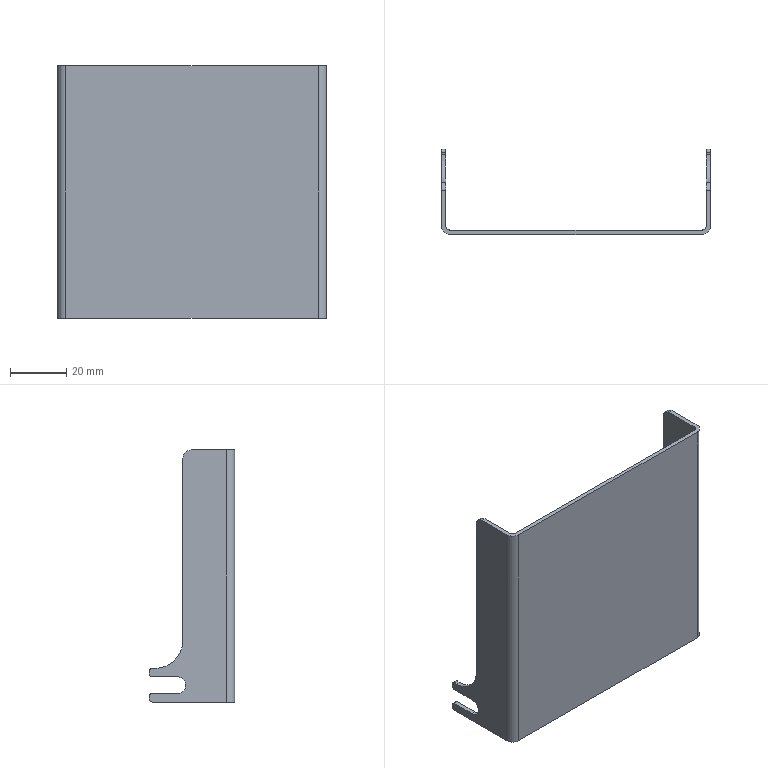Part | NX | features BREP 1 | 1 solid | 38 faces | box 96 x 30.5 x 90 mm | volume 17555 mm3 | plane 20 | cylinder 18 | commonest cylinder face diameters 2 x8 6 x6 3 x2 20 x2
STEP:
#1=CARTESIAN_POINT('',(-45.,0.,90.));
#2=VERTEX_POINT('',#1);
#3=CARTESIAN_POINT('',(45.,0.,90.));
#4=VERTEX_POINT('',#3);
#5=CARTESIAN_POINT('',(-46.5,0.,90.));
#6=DIRECTION('',(1.,0.,0.));
#7=VECTOR('',#6,1000.);
#8=LINE('',#5,#7);
#9=EDGE_CURVE('',#2,#4,#8,.T.);
#10=ORIENTED_EDGE('',*,*,#9,.T.);
#11=CARTESIAN_POINT('',(45.,0.,0.));
#12=VERTEX_POINT('',#11);
#13=CARTESIAN_POINT('',(45.,0.,90.));
#14=DIRECTION('',(0.,0.,-1.));
#15=VECTOR('',#14,1000.);
#16=LINE('',#13,#15);
#17=EDGE_CURVE('',#4,#12,#16,.T.);
#18=ORIENTED_EDGE('',*,*,#17,.T.);
#19=CARTESIAN_POINT('',(-45.,0.,0.));
#20=VERTEX_POINT('',#19);
#21=CARTESIAN_POINT('',(-46.5,0.,0.));
#22=DIRECTION('',(-1.,0.,0.));
#23=VECTOR('',#22,1000.);
#24=LINE('',#21,#23);
#25=EDGE_CURVE('',#12,#20,#24,.T.);
#26=ORIENTED_EDGE('',*,*,#25,.T.);
#27=CARTESIAN_POINT('',(-45.,0.,90.));
#28=DIRECTION('',(0.,0.,1.));
#29=VECTOR('',#28,1000.);
#30=LINE('',#27,#29);
#31=EDGE_CURVE('',#20,#2,#30,.T.);
#32=ORIENTED_EDGE('',*,*,#31,.T.);
#33=EDGE_LOOP('',(#10,#18,#26,#32));
#34=FACE_BOUND('',#33,.T.);
#35=CARTESIAN_POINT('',(-46.5,0.,90.));
#36=DIRECTION('',(0.,1.,0.));
#37=DIRECTION('',(1.,0.,0.));
#38=AXIS2_PLACEMENT_3D('',#35,#36,#37);
#39=PLANE('',#38);
#40=ADVANCED_FACE('',(#34),#39,.T.);
#41=ORIENTED_EDGE('',*,*,#17,.F.);
#42=CARTESIAN_POINT('',(46.5,1.5,90.));
#43=VERTEX_POINT('',#42);
#44=CARTESIAN_POINT('',(45.,1.5,90.));
#45=DIRECTION('',(0.,0.,-1.));
#46=DIRECTION('',(-1.,0.,0.));
#47=AXIS2_PLACEMENT_3D('',#44,#45,#46);
#48=CIRCLE('',#47,1.5);
#49=EDGE_CURVE('',#43,#4,#48,.T.);
#50=ORIENTED_EDGE('',*,*,#49,.F.);
#51=CARTESIAN_POINT('',(46.5,1.5,0.));
#52=VERTEX_POINT('',#51);
#53=CARTESIAN_POINT('',(46.5,1.5,90.));
#54=DIRECTION('',(0.,0.,1.));
#55=VECTOR('',#54,1000.);
#56=LINE('',#53,#55);
#57=EDGE_CURVE('',#52,#43,#56,.T.);
#58=ORIENTED_EDGE('',*,*,#57,.F.);
#59=CARTESIAN_POINT('',(45.,1.5,0.));
#60=DIRECTION('',(0.,0.,1.));
#61=DIRECTION('',(-1.,0.,0.));
#62=AXIS2_PLACEMENT_3D('',#59,#60,#61);
#63=CIRCLE('',#62,1.5);
#64=EDGE_CURVE('',#12,#52,#63,.T.);
#65=ORIENTED_EDGE('',*,*,#64,.F.);
#66=EDGE_LOOP('',(#41,#50,#58,#65));
#67=FACE_BOUND('',#66,.T.);
#68=CARTESIAN_POINT('',(45.,1.5,90.));
#69=DIRECTION('',(0.,0.,-1.));
#70=DIRECTION('',(1.,0.,0.));
#71=AXIS2_PLACEMENT_3D('',#68,#69,#70);
#72=CYLINDRICAL_SURFACE('',#71,1.5);
#73=ADVANCED_FACE('',(#67),#72,.F.);
#74=CARTESIAN_POINT('',(-45.,-1.5,90.));
#75=VERTEX_POINT('',#74);
#76=CARTESIAN_POINT('',(45.,-1.5,90.));
#77=VERTEX_POINT('',#76);
#78=CARTESIAN_POINT('',(-48.,-1.5,90.));
#79=DIRECTION('',(1.,0.,0.));
#80=VECTOR('',#79,1000.);
#81=LINE('',#78,#80);
#82=EDGE_CURVE('',#75,#77,#81,.T.);
#83=ORIENTED_EDGE('',*,*,#82,.T.);
#84=CARTESIAN_POINT('',(48.,1.5,90.));
#85=VERTEX_POINT('',#84);
#86=CARTESIAN_POINT('',(45.,1.5,90.));
#87=DIRECTION('',(0.,0.,1.));
#88=DIRECTION('',(-1.,0.,0.));
#89=AXIS2_PLACEMENT_3D('',#86,#87,#88);
#90=CIRCLE('',#89,3.);
#91=EDGE_CURVE('',#77,#85,#90,.T.);
#92=ORIENTED_EDGE('',*,*,#91,.T.);
#93=CARTESIAN_POINT('',(48.,14.,90.));
#94=VERTEX_POINT('',#93);
#95=CARTESIAN_POINT('',(48.,-1.5,90.));
#96=DIRECTION('',(0.,1.,0.));
#97=VECTOR('',#96,1000.);
#98=LINE('',#95,#97);
#99=EDGE_CURVE('',#85,#94,#98,.T.);
#100=ORIENTED_EDGE('',*,*,#99,.T.);
#101=CARTESIAN_POINT('',(46.5,14.,90.));
#102=VERTEX_POINT('',#101);
#103=CARTESIAN_POINT('',(46.5,14.,90.));
#104=DIRECTION('',(1.,0.,0.));
#105=VECTOR('',#104,1000.);
#106=LINE('',#103,#105);
#107=EDGE_CURVE('',#102,#94,#106,.T.);
#108=ORIENTED_EDGE('',*,*,#107,.F.);
#109=CARTESIAN_POINT('',(46.5,0.,90.));
#110=DIRECTION('',(0.,1.,0.));
#111=VECTOR('',#110,1000.);
#112=LINE('',#109,#111);
#113=EDGE_CURVE('',#43,#102,#112,.T.);
#114=ORIENTED_EDGE('',*,*,#113,.F.);
#115=ORIENTED_EDGE('',*,*,#49,.T.);
#116=ORIENTED_EDGE('',*,*,#9,.F.);
#117=CARTESIAN_POINT('',(-46.5,1.5,90.));
#118=VERTEX_POINT('',#117);
#119=CARTESIAN_POINT('',(-45.,1.5,90.));
#120=DIRECTION('',(0.,0.,-1.));
#121=DIRECTION('',(-1.,0.,0.));
#122=AXIS2_PLACEMENT_3D('',#119,#120,#121);
#123=CIRCLE('',#122,1.5);
#124=EDGE_CURVE('',#2,#118,#123,.T.);
#125=ORIENTED_EDGE('',*,*,#124,.T.);
#126=CARTESIAN_POINT('',(-46.5,14.,90.));
#127=VERTEX_POINT('',#126);
#128=CARTESIAN_POINT('',(-46.5,17.,90.));
#129=DIRECTION('',(0.,-1.,0.));
#130=VECTOR('',#129,1000.);
#131=LINE('',#128,#130);
#132=EDGE_CURVE('',#127,#118,#131,.T.);
#133=ORIENTED_EDGE('',*,*,#132,.F.);
#134=CARTESIAN_POINT('',(-48.,14.,90.));
#135=VERTEX_POINT('',#134);
#136=CARTESIAN_POINT('',(45.,14.,90.));
#137=DIRECTION('',(1.,0.,0.));
#138=VECTOR('',#137,1000.);
#139=LINE('',#136,#138);
#140=EDGE_CURVE('',#135,#127,#139,.T.);
#141=ORIENTED_EDGE('',*,*,#140,.F.);
#142=CARTESIAN_POINT('',(-48.,1.5,90.));
#143=VERTEX_POINT('',#142);
#144=CARTESIAN_POINT('',(-48.,1.5,90.));
#145=DIRECTION('',(0.,1.,0.));
#146=VECTOR('',#145,1000.);
#147=LINE('',#144,#146);
#148=EDGE_CURVE('',#143,#135,#147,.T.);
#149=ORIENTED_EDGE('',*,*,#148,.F.);
#150=CARTESIAN_POINT('',(-45.,1.5,90.));
#151=DIRECTION('',(0.,0.,1.));
#152=DIRECTION('',(-1.,0.,0.));
#153=AXIS2_PLACEMENT_3D('',#150,#151,#152);
#154=CIRCLE('',#153,3.);
#155=EDGE_CURVE('',#143,#75,#154,.T.);
#156=ORIENTED_EDGE('',*,*,#155,.T.);
#157=EDGE_LOOP('',(#83,#92,#100,#108,#114,#115,#116,#125,#133,#141,#149,#156));
#158=FACE_BOUND('',#157,.T.);
#159=CARTESIAN_POINT('',(-48.,1.5,90.));
#160=DIRECTION('',(0.,0.,1.));
#161=DIRECTION('',(-1.,0.,0.));
#162=AXIS2_PLACEMENT_3D('',#159,#160,#161);
#163=PLANE('',#162);
#164=ADVANCED_FACE('',(#158),#163,.T.);
#165=CARTESIAN_POINT('',(-46.5,1.5,0.));
#166=VERTEX_POINT('',#165);
#167=CARTESIAN_POINT('',(-46.5,1.5,90.));
#168=DIRECTION('',(0.,0.,-1.));
#169=VECTOR('',#168,1000.);
#170=LINE('',#167,#169);
#171=EDGE_CURVE('',#118,#166,#170,.T.);
#172=ORIENTED_EDGE('',*,*,#171,.F.);
#173=ORIENTED_EDGE('',*,*,#124,.F.);
#174=ORIENTED_EDGE('',*,*,#31,.F.);
#175=CARTESIAN_POINT('',(-45.,1.5,0.));
#176=DIRECTION('',(0.,0.,1.));
#177=DIRECTION('',(-1.,0.,0.));
#178=AXIS2_PLACEMENT_3D('',#175,#176,#177);
#179=CIRCLE('',#178,1.5);
#180=EDGE_CURVE('',#166,#20,#179,.T.);
#181=ORIENTED_EDGE('',*,*,#180,.F.);
#182=EDGE_LOOP('',(#172,#173,#174,#181));
#183=FACE_BOUND('',#182,.T.);
#184=CARTESIAN_POINT('',(-45.,1.5,90.));
#185=DIRECTION('',(0.,0.,-1.));
#186=DIRECTION('',(1.,0.,0.));
#187=AXIS2_PLACEMENT_3D('',#184,#185,#186);
#188=CYLINDRICAL_SURFACE('',#187,1.5);
#189=ADVANCED_FACE('',(#183),#188,.F.);
#190=CARTESIAN_POINT('',(45.,-1.5,0.));
#191=VERTEX_POINT('',#190);
#192=CARTESIAN_POINT('',(-45.,-1.5,0.));
#193=VERTEX_POINT('',#192);
#194=CARTESIAN_POINT('',(48.,-1.5,0.));
#195=DIRECTION('',(-1.,0.,0.));
#196=VECTOR('',#195,1000.);
#197=LINE('',#194,#196);
#198=EDGE_CURVE('',#191,#193,#197,.T.);
#199=ORIENTED_EDGE('',*,*,#198,.T.);
#200=CARTESIAN_POINT('',(-48.,1.5,0.));
#201=VERTEX_POINT('',#200);
#202=CARTESIAN_POINT('',(-45.,1.5,0.));
#203=DIRECTION('',(0.,0.,-1.));
#204=DIRECTION('',(-1.,0.,0.));
#205=AXIS2_PLACEMENT_3D('',#202,#203,#204);
#206=CIRCLE('',#205,3.);
#207=EDGE_CURVE('',#193,#201,#206,.T.);
#208=ORIENTED_EDGE('',*,*,#207,.T.);
#209=CARTESIAN_POINT('',(-48.,28.,0.));
#210=VERTEX_POINT('',#209);
#211=CARTESIAN_POINT('',(-48.,-1.5,0.));
#212=DIRECTION('',(0.,1.,0.));
#213=VECTOR('',#212,1000.);
#214=LINE('',#211,#213);
#215=EDGE_CURVE('',#201,#210,#214,.T.);
#216=ORIENTED_EDGE('',*,*,#215,.T.);
#217=CARTESIAN_POINT('',(-46.5,28.,0.));
#218=VERTEX_POINT('',#217);
#219=CARTESIAN_POINT('',(-29.529,28.,0.));
#220=DIRECTION('',(-1.,0.,0.));
#221=VECTOR('',#220,1000.);
#222=LINE('',#219,#221);
#223=EDGE_CURVE('',#218,#210,#222,.T.);
#224=ORIENTED_EDGE('',*,*,#223,.F.);
#225=CARTESIAN_POINT('',(-46.5,17.,0.));
#226=DIRECTION('',(0.,1.,0.));
#227=VECTOR('',#226,1000.);
#228=LINE('',#225,#227);
#229=EDGE_CURVE('',#166,#218,#228,.T.);
#230=ORIENTED_EDGE('',*,*,#229,.F.);
#231=ORIENTED_EDGE('',*,*,#180,.T.);
#232=ORIENTED_EDGE('',*,*,#25,.F.);
#233=ORIENTED_EDGE('',*,*,#64,.T.);
#234=CARTESIAN_POINT('',(46.5,28.,0.));
#235=VERTEX_POINT('',#234);
#236=CARTESIAN_POINT('',(46.5,0.,0.));
#237=DIRECTION('',(0.,-1.,0.));
#238=VECTOR('',#237,1000.);
#239=LINE('',#236,#238);
#240=EDGE_CURVE('',#235,#52,#239,.T.);
#241=ORIENTED_EDGE('',*,*,#240,.F.);
#242=CARTESIAN_POINT('',(48.,28.,0.));
#243=VERTEX_POINT('',#242);
#244=CARTESIAN_POINT('',(45.,28.,0.));
#245=DIRECTION('',(1.,0.,0.));
#246=VECTOR('',#245,1000.);
#247=LINE('',#244,#246);
#248=EDGE_CURVE('',#235,#243,#247,.T.);
#249=ORIENTED_EDGE('',*,*,#248,.T.);
#250=CARTESIAN_POINT('',(48.,1.5,0.));
#251=VERTEX_POINT('',#250);
#252=CARTESIAN_POINT('',(48.,1.5,0.));
#253=DIRECTION('',(0.,-1.,0.));
#254=VECTOR('',#253,1000.);
#255=LINE('',#252,#254);
#256=EDGE_CURVE('',#243,#251,#255,.T.);
#257=ORIENTED_EDGE('',*,*,#256,.T.);
#258=CARTESIAN_POINT('',(45.,1.5,0.));
#259=DIRECTION('',(0.,0.,-1.));
#260=DIRECTION('',(-1.,0.,0.));
#261=AXIS2_PLACEMENT_3D('',#258,#259,#260);
#262=CIRCLE('',#261,3.);
#263=EDGE_CURVE('',#251,#191,#262,.T.);
#264=ORIENTED_EDGE('',*,*,#263,.T.);
#265=EDGE_LOOP('',(#199,#208,#216,#224,#230,#231,#232,#233,#241,#249,#257,#264));
#266=FACE_BOUND('',#265,.T.);
#267=CARTESIAN_POINT('',(48.,1.5,0.));
#268=DIRECTION('',(0.,0.,-1.));
#269=DIRECTION('',(1.,0.,0.));
#270=AXIS2_PLACEMENT_3D('',#267,#268,#269);
#271=PLANE('',#270);
#272=ADVANCED_FACE('',(#266),#271,.T.);
#273=CARTESIAN_POINT('',(46.5,27.,12.));
#274=VERTEX_POINT('',#273);
#275=CARTESIAN_POINT('',(46.5,28.,12.));
#276=VERTEX_POINT('',#275);
#277=CARTESIAN_POINT('',(46.5,0.,12.));
#278=DIRECTION('',(0.,1.,0.));
#279=VECTOR('',#278,1000.);
#280=LINE('',#277,#279);
#281=EDGE_CURVE('',#274,#276,#280,.T.);
#282=ORIENTED_EDGE('',*,*,#281,.T.);
#283=CARTESIAN_POINT('',(46.5,29.,11.));
#284=VERTEX_POINT('',#283);
#285=CARTESIAN_POINT('',(46.5,28.,11.));
#286=DIRECTION('',(-1.,0.,0.));
#287=DIRECTION('',(0.,0.,-1.));
#288=AXIS2_PLACEMENT_3D('',#285,#286,#287);
#289=CIRCLE('',#288,1.);
#290=EDGE_CURVE('',#276,#284,#289,.T.);
#291=ORIENTED_EDGE('',*,*,#290,.T.);
#292=CARTESIAN_POINT('',(46.5,29.,10.));
#293=VERTEX_POINT('',#292);
#294=CARTESIAN_POINT('',(46.5,29.,90.));
#295=DIRECTION('',(0.,0.,-1.));
#296=VECTOR('',#295,1000.);
#297=LINE('',#294,#296);
#298=EDGE_CURVE('',#284,#293,#297,.T.);
#299=ORIENTED_EDGE('',*,*,#298,.T.);
#300=CARTESIAN_POINT('',(46.5,28.,9.));
#301=VERTEX_POINT('',#300);
#302=CARTESIAN_POINT('',(46.5,28.,10.));
#303=DIRECTION('',(-1.,0.,0.));
#304=DIRECTION('',(0.,0.,1.));
#305=AXIS2_PLACEMENT_3D('',#302,#303,#304);
#306=CIRCLE('',#305,1.);
#307=EDGE_CURVE('',#293,#301,#306,.T.);
#308=ORIENTED_EDGE('',*,*,#307,.T.);
#309=CARTESIAN_POINT('',(46.5,19.,9.));
#310=VERTEX_POINT('',#309);
#311=CARTESIAN_POINT('',(46.5,0.,9.));
#312=DIRECTION('',(0.,-1.,0.));
#313=VECTOR('',#312,1000.);
#314=LINE('',#311,#313);
#315=EDGE_CURVE('',#301,#310,#314,.T.);
#316=ORIENTED_EDGE('',*,*,#315,.T.);
#317=CARTESIAN_POINT('',(46.5,19.,3.));
#318=VERTEX_POINT('',#317);
#319=CARTESIAN_POINT('',(46.5,19.,6.));
#320=DIRECTION('',(1.,0.,0.));
#321=DIRECTION('',(0.,0.,-1.));
#322=AXIS2_PLACEMENT_3D('',#319,#320,#321);
#323=CIRCLE('',#322,3.);
#324=EDGE_CURVE('',#310,#318,#323,.T.);
#325=ORIENTED_EDGE('',*,*,#324,.T.);
#326=CARTESIAN_POINT('',(46.5,28.,3.));
#327=VERTEX_POINT('',#326);
#328=CARTESIAN_POINT('',(46.5,0.,3.));
#329=DIRECTION('',(0.,1.,0.));
#330=VECTOR('',#329,1000.);
#331=LINE('',#328,#330);
#332=EDGE_CURVE('',#318,#327,#331,.T.);
#333=ORIENTED_EDGE('',*,*,#332,.T.);
#334=CARTESIAN_POINT('',(46.5,29.,2.));
#335=VERTEX_POINT('',#334);
#336=CARTESIAN_POINT('',(46.5,28.,2.));
#337=DIRECTION('',(-1.,0.,0.));
#338=DIRECTION('',(0.,0.,-1.));
#339=AXIS2_PLACEMENT_3D('',#336,#337,#338);
#340=CIRCLE('',#339,1.);
#341=EDGE_CURVE('',#327,#335,#340,.T.);
#342=ORIENTED_EDGE('',*,*,#341,.T.);
#343=CARTESIAN_POINT('',(46.5,29.,1.));
#344=VERTEX_POINT('',#343);
#345=CARTESIAN_POINT('',(46.5,29.,90.));
#346=DIRECTION('',(0.,0.,-1.));
#347=VECTOR('',#346,1000.);
#348=LINE('',#345,#347);
#349=EDGE_CURVE('',#335,#344,#348,.T.);
#350=ORIENTED_EDGE('',*,*,#349,.T.);
#351=CARTESIAN_POINT('',(46.5,28.,1.));
#352=DIRECTION('',(-1.,0.,0.));
#353=DIRECTION('',(0.,0.,-1.));
#354=AXIS2_PLACEMENT_3D('',#351,#352,#353);
#355=CIRCLE('',#354,1.);
#356=EDGE_CURVE('',#344,#235,#355,.T.);
#357=ORIENTED_EDGE('',*,*,#356,.T.);
#358=ORIENTED_EDGE('',*,*,#240,.T.);
#359=ORIENTED_EDGE('',*,*,#57,.T.);
#360=ORIENTED_EDGE('',*,*,#113,.T.);
#361=CARTESIAN_POINT('',(46.5,17.,87.));
#362=VERTEX_POINT('',#361);
#363=CARTESIAN_POINT('',(46.5,14.,87.));
#364=DIRECTION('',(-1.,0.,0.));
#365=DIRECTION('',(0.,0.,-1.));
#366=AXIS2_PLACEMENT_3D('',#363,#364,#365);
#367=CIRCLE('',#366,3.);
#368=EDGE_CURVE('',#102,#362,#367,.T.);
#369=ORIENTED_EDGE('',*,*,#368,.T.);
#370=CARTESIAN_POINT('',(46.5,17.,22.));
#371=VERTEX_POINT('',#370);
#372=CARTESIAN_POINT('',(46.5,17.,90.));
#373=DIRECTION('',(0.,0.,-1.));
#374=VECTOR('',#373,1000.);
#375=LINE('',#372,#374);
#376=EDGE_CURVE('',#362,#371,#375,.T.);
#377=ORIENTED_EDGE('',*,*,#376,.T.);
#378=CARTESIAN_POINT('',(46.5,27.,22.));
#379=DIRECTION('',(1.,0.,0.));
#380=DIRECTION('',(0.,0.,1.));
#381=AXIS2_PLACEMENT_3D('',#378,#379,#380);
#382=CIRCLE('',#381,10.);
#383=EDGE_CURVE('',#371,#274,#382,.T.);
#384=ORIENTED_EDGE('',*,*,#383,.T.);
#385=EDGE_LOOP('',(#282,#291,#299,#308,#316,#325,#333,#342,#350,#357,#358,#359,#360,#369,#377,#384));
#386=FACE_BOUND('',#385,.T.);
#387=CARTESIAN_POINT('',(46.5,0.,90.));
#388=DIRECTION('',(-1.,0.,0.));
#389=DIRECTION('',(0.,0.,-1.));
#390=AXIS2_PLACEMENT_3D('',#387,#388,#389);
#391=PLANE('',#390);
#392=ADVANCED_FACE('',(#386),#391,.T.);
#393=CARTESIAN_POINT('',(45.,-1.5,90.));
#394=DIRECTION('',(0.,0.,-1.));
#395=VECTOR('',#394,1000.);
#396=LINE('',#393,#395);
#397=EDGE_CURVE('',#77,#191,#396,.T.);
#398=ORIENTED_EDGE('',*,*,#397,.F.);
#399=ORIENTED_EDGE('',*,*,#82,.F.);
#400=CARTESIAN_POINT('',(-45.,-1.5,90.));
#401=DIRECTION('',(0.,0.,1.));
#402=VECTOR('',#401,1000.);
#403=LINE('',#400,#402);
#404=EDGE_CURVE('',#193,#75,#403,.T.);
#405=ORIENTED_EDGE('',*,*,#404,.F.);
#406=ORIENTED_EDGE('',*,*,#198,.F.);
#407=EDGE_LOOP('',(#398,#399,#405,#406));
#408=FACE_BOUND('',#407,.T.);
#409=CARTESIAN_POINT('',(-46.5,-1.5,90.));
#410=DIRECTION('',(0.,1.,0.));
#411=DIRECTION('',(1.,0.,0.));
#412=AXIS2_PLACEMENT_3D('',#409,#410,#411);
#413=PLANE('',#412);
#414=ADVANCED_FACE('',(#408),#413,.F.);
#415=ORIENTED_EDGE('',*,*,#229,.T.);
#416=CARTESIAN_POINT('',(-46.5,29.,1.));
#417=VERTEX_POINT('',#416);
#418=CARTESIAN_POINT('',(-46.5,28.,1.));
#419=DIRECTION('',(1.,0.,0.));
#420=DIRECTION('',(0.,0.,1.));
#421=AXIS2_PLACEMENT_3D('',#418,#419,#420);
#422=CIRCLE('',#421,1.);
#423=EDGE_CURVE('',#218,#417,#422,.T.);
#424=ORIENTED_EDGE('',*,*,#423,.T.);
#425=CARTESIAN_POINT('',(-46.5,29.,2.));
#426=VERTEX_POINT('',#425);
#427=CARTESIAN_POINT('',(-46.5,29.,90.));
#428=DIRECTION('',(0.,0.,1.));
#429=VECTOR('',#428,1000.);
#430=LINE('',#427,#429);
#431=EDGE_CURVE('',#417,#426,#430,.T.);
#432=ORIENTED_EDGE('',*,*,#431,.T.);
#433=CARTESIAN_POINT('',(-46.5,28.,3.));
#434=VERTEX_POINT('',#433);
#435=CARTESIAN_POINT('',(-46.5,28.,2.));
#436=DIRECTION('',(1.,0.,0.));
#437=DIRECTION('',(0.,0.,1.));
#438=AXIS2_PLACEMENT_3D('',#435,#436,#437);
#439=CIRCLE('',#438,1.);
#440=EDGE_CURVE('',#426,#434,#439,.T.);
#441=ORIENTED_EDGE('',*,*,#440,.T.);
#442=CARTESIAN_POINT('',(-46.5,19.,3.));
#443=VERTEX_POINT('',#442);
#444=CARTESIAN_POINT('',(-46.5,17.,3.));
#445=DIRECTION('',(0.,-1.,0.));
#446=VECTOR('',#445,1000.);
#447=LINE('',#444,#446);
#448=EDGE_CURVE('',#434,#443,#447,.T.);
#449=ORIENTED_EDGE('',*,*,#448,.T.);
#450=CARTESIAN_POINT('',(-46.5,19.,9.));
#451=VERTEX_POINT('',#450);
#452=CARTESIAN_POINT('',(-46.5,19.,6.));
#453=DIRECTION('',(-1.,0.,0.));
#454=DIRECTION('',(0.,0.,-1.));
#455=AXIS2_PLACEMENT_3D('',#452,#453,#454);
#456=CIRCLE('',#455,3.);
#457=EDGE_CURVE('',#443,#451,#456,.T.);
#458=ORIENTED_EDGE('',*,*,#457,.T.);
#459=CARTESIAN_POINT('',(-46.5,28.,9.));
#460=VERTEX_POINT('',#459);
#461=CARTESIAN_POINT('',(-46.5,17.,9.));
#462=DIRECTION('',(0.,1.,0.));
#463=VECTOR('',#462,1000.);
#464=LINE('',#461,#463);
#465=EDGE_CURVE('',#451,#460,#464,.T.);
#466=ORIENTED_EDGE('',*,*,#465,.T.);
#467=CARTESIAN_POINT('',(-46.5,29.,10.));
#468=VERTEX_POINT('',#467);
#469=CARTESIAN_POINT('',(-46.5,28.,10.));
#470=DIRECTION('',(1.,0.,0.));
#471=DIRECTION('',(0.,0.,1.));
#472=AXIS2_PLACEMENT_3D('',#469,#470,#471);
#473=CIRCLE('',#472,1.);
#474=EDGE_CURVE('',#460,#468,#473,.T.);
#475=ORIENTED_EDGE('',*,*,#474,.T.);
#476=CARTESIAN_POINT('',(-46.5,29.,11.));
#477=VERTEX_POINT('',#476);
#478=CARTESIAN_POINT('',(-46.5,29.,90.));
#479=DIRECTION('',(0.,0.,1.));
#480=VECTOR('',#479,1000.);
#481=LINE('',#478,#480);
#482=EDGE_CURVE('',#468,#477,#481,.T.);
#483=ORIENTED_EDGE('',*,*,#482,.T.);
#484=CARTESIAN_POINT('',(-46.5,28.,12.));
#485=VERTEX_POINT('',#484);
#486=CARTESIAN_POINT('',(-46.5,28.,11.));
#487=DIRECTION('',(1.,0.,0.));
#488=DIRECTION('',(0.,0.,1.));
#489=AXIS2_PLACEMENT_3D('',#486,#487,#488);
#490=CIRCLE('',#489,1.);
#491=EDGE_CURVE('',#477,#485,#490,.T.);
#492=ORIENTED_EDGE('',*,*,#491,.T.);
#493=CARTESIAN_POINT('',(-46.5,27.,12.));
#494=VERTEX_POINT('',#493);
#495=CARTESIAN_POINT('',(-46.5,17.,12.));
#496=DIRECTION('',(0.,-1.,0.));
#497=VECTOR('',#496,1000.);
#498=LINE('',#495,#497);
#499=EDGE_CURVE('',#485,#494,#498,.T.);
#500=ORIENTED_EDGE('',*,*,#499,.T.);
#501=CARTESIAN_POINT('',(-46.5,17.,22.));
#502=VERTEX_POINT('',#501);
#503=CARTESIAN_POINT('',(-46.5,27.,22.));
#504=DIRECTION('',(-1.,0.,0.));
#505=DIRECTION('',(0.,0.,-1.));
#506=AXIS2_PLACEMENT_3D('',#503,#504,#505);
#507=CIRCLE('',#506,10.);
#508=EDGE_CURVE('',#494,#502,#507,.T.);
#509=ORIENTED_EDGE('',*,*,#508,.T.);
#510=CARTESIAN_POINT('',(-46.5,17.,87.));
#511=VERTEX_POINT('',#510);
#512=CARTESIAN_POINT('',(-46.5,17.,90.));
#513=DIRECTION('',(0.,0.,1.));
#514=VECTOR('',#513,1000.);
#515=LINE('',#512,#514);
#516=EDGE_CURVE('',#502,#511,#515,.T.);
#517=ORIENTED_EDGE('',*,*,#516,.T.);
#518=CARTESIAN_POINT('',(-46.5,14.,87.));
#519=DIRECTION('',(1.,0.,0.));
#520=DIRECTION('',(0.,0.,1.));
#521=AXIS2_PLACEMENT_3D('',#518,#519,#520);
#522=CIRCLE('',#521,3.);
#523=EDGE_CURVE('',#511,#127,#522,.T.);
#524=ORIENTED_EDGE('',*,*,#523,.T.);
#525=ORIENTED_EDGE('',*,*,#132,.T.);
#526=ORIENTED_EDGE('',*,*,#171,.T.);
#527=EDGE_LOOP('',(#415,#424,#432,#441,#449,#458,#466,#475,#483,#492,#500,#509,#517,#524,#525,#526));
#528=FACE_BOUND('',#527,.T.);
#529=CARTESIAN_POINT('',(-46.5,17.,90.));
#530=DIRECTION('',(1.,0.,0.));
#531=DIRECTION('',(0.,0.,1.));
#532=AXIS2_PLACEMENT_3D('',#529,#530,#531);
#533=PLANE('',#532);
#534=ADVANCED_FACE('',(#528),#533,.T.);
#535=ORIENTED_EDGE('',*,*,#91,.F.);
#536=ORIENTED_EDGE('',*,*,#397,.T.);
#537=ORIENTED_EDGE('',*,*,#263,.F.);
#538=CARTESIAN_POINT('',(48.,1.5,90.));
#539=DIRECTION('',(0.,0.,1.));
#540=VECTOR('',#539,1000.);
#541=LINE('',#538,#540);
#542=EDGE_CURVE('',#251,#85,#541,.T.);
#543=ORIENTED_EDGE('',*,*,#542,.T.);
#544=EDGE_LOOP('',(#535,#536,#537,#543));
#545=FACE_BOUND('',#544,.T.);
#546=CARTESIAN_POINT('',(45.,1.5,90.));
#547=DIRECTION('',(0.,0.,-1.));
#548=DIRECTION('',(1.,0.,0.));
#549=AXIS2_PLACEMENT_3D('',#546,#547,#548);
#550=CYLINDRICAL_SURFACE('',#549,3.);
#551=ADVANCED_FACE('',(#545),#550,.T.);
#552=CARTESIAN_POINT('',(48.,28.,12.));
#553=VERTEX_POINT('',#552);
#554=CARTESIAN_POINT('',(48.,29.,11.));
#555=VERTEX_POINT('',#554);
#556=CARTESIAN_POINT('',(48.,28.,11.));
#557=DIRECTION('',(-1.,0.,0.));
#558=DIRECTION('',(0.,0.,-1.));
#559=AXIS2_PLACEMENT_3D('',#556,#557,#558);
#560=CIRCLE('',#559,1.);
#561=EDGE_CURVE('',#553,#555,#560,.T.);
#562=ORIENTED_EDGE('',*,*,#561,.T.);
#563=CARTESIAN_POINT('',(46.5,29.,11.));
#564=DIRECTION('',(-1.,0.,0.));
#565=VECTOR('',#564,1000.);
#566=LINE('',#563,#565);
#567=EDGE_CURVE('',#555,#284,#566,.T.);
#568=ORIENTED_EDGE('',*,*,#567,.T.);
#569=ORIENTED_EDGE('',*,*,#290,.F.);
#570=CARTESIAN_POINT('',(46.5,28.,12.));
#571=DIRECTION('',(1.,0.,0.));
#572=VECTOR('',#571,1000.);
#573=LINE('',#570,#572);
#574=EDGE_CURVE('',#276,#553,#573,.T.);
#575=ORIENTED_EDGE('',*,*,#574,.T.);
#576=EDGE_LOOP('',(#562,#568,#569,#575));
#577=FACE_BOUND('',#576,.T.);
#578=CARTESIAN_POINT('',(46.5,28.,11.));
#579=DIRECTION('',(1.,0.,0.));
#580=DIRECTION('',(0.,0.,1.));
#581=AXIS2_PLACEMENT_3D('',#578,#579,#580);
#582=CYLINDRICAL_SURFACE('',#581,1.);
#583=ADVANCED_FACE('',(#577),#582,.T.);
#584=ORIENTED_EDGE('',*,*,#281,.F.);
#585=CARTESIAN_POINT('',(48.,27.,12.));
#586=VERTEX_POINT('',#585);
#587=CARTESIAN_POINT('',(46.5,27.,12.));
#588=DIRECTION('',(1.,0.,0.));
#589=VECTOR('',#588,1000.);
#590=LINE('',#587,#589);
#591=EDGE_CURVE('',#274,#586,#590,.T.);
#592=ORIENTED_EDGE('',*,*,#591,.T.);
#593=CARTESIAN_POINT('',(48.,29.,12.));
#594=DIRECTION('',(0.,1.,0.));
#595=VECTOR('',#594,1000.);
#596=LINE('',#593,#595);
#597=EDGE_CURVE('',#586,#553,#596,.T.);
#598=ORIENTED_EDGE('',*,*,#597,.T.);
#599=ORIENTED_EDGE('',*,*,#574,.F.);
#600=EDGE_LOOP('',(#584,#592,#598,#599));
#601=FACE_BOUND('',#600,.T.);
#602=CARTESIAN_POINT('',(46.5,29.,12.));
#603=DIRECTION('',(0.,0.,1.));
#604=DIRECTION('',(0.,1.,0.));
#605=AXIS2_PLACEMENT_3D('',#602,#603,#604);
#606=PLANE('',#605);
#607=ADVANCED_FACE('',(#601),#606,.T.);
#608=CARTESIAN_POINT('',(48.,17.,22.));
#609=VERTEX_POINT('',#608);
#610=CARTESIAN_POINT('',(46.5,17.,22.));
#611=DIRECTION('',(-1.,0.,0.));
#612=VECTOR('',#611,1000.);
#613=LINE('',#610,#612);
#614=EDGE_CURVE('',#609,#371,#613,.T.);
#615=ORIENTED_EDGE('',*,*,#614,.F.);
#616=CARTESIAN_POINT('',(48.,27.,22.));
#617=DIRECTION('',(-1.,0.,0.));
#618=DIRECTION('',(0.,0.,1.));
#619=AXIS2_PLACEMENT_3D('',#616,#617,#618);
#620=CIRCLE('',#619,10.);
#621=EDGE_CURVE('',#586,#609,#620,.T.);
#622=ORIENTED_EDGE('',*,*,#621,.F.);
#623=ORIENTED_EDGE('',*,*,#591,.F.);
#624=ORIENTED_EDGE('',*,*,#383,.F.);
#625=EDGE_LOOP('',(#615,#622,#623,#624));
#626=FACE_BOUND('',#625,.T.);
#627=CARTESIAN_POINT('',(46.5,27.,22.));
#628=DIRECTION('',(-1.,0.,0.));
#629=DIRECTION('',(0.,0.,-1.));
#630=AXIS2_PLACEMENT_3D('',#627,#628,#629);
#631=CYLINDRICAL_SURFACE('',#630,10.);
#632=ADVANCED_FACE('',(#626),#631,.F.);
#633=CARTESIAN_POINT('',(48.,17.,87.));
#634=VERTEX_POINT('',#633);
#635=CARTESIAN_POINT('',(48.,17.,90.));
#636=DIRECTION('',(0.,0.,-1.));
#637=VECTOR('',#636,1000.);
#638=LINE('',#635,#637);
#639=EDGE_CURVE('',#634,#609,#638,.T.);
#640=ORIENTED_EDGE('',*,*,#639,.T.);
#641=ORIENTED_EDGE('',*,*,#614,.T.);
#642=ORIENTED_EDGE('',*,*,#376,.F.);
#643=CARTESIAN_POINT('',(46.5,17.,87.));
#644=DIRECTION('',(1.,0.,0.));
#645=VECTOR('',#644,1000.);
#646=LINE('',#643,#645);
#647=EDGE_CURVE('',#362,#634,#646,.T.);
#648=ORIENTED_EDGE('',*,*,#647,.T.);
#649=EDGE_LOOP('',(#640,#641,#642,#648));
#650=FACE_BOUND('',#649,.T.);
#651=CARTESIAN_POINT('',(46.5,17.,90.));
#652=DIRECTION('',(0.,1.,0.));
#653=DIRECTION('',(0.,0.,-1.));
#654=AXIS2_PLACEMENT_3D('',#651,#652,#653);
#655=PLANE('',#654);
#656=ADVANCED_FACE('',(#650),#655,.T.);
#657=CARTESIAN_POINT('',(48.,14.,87.));
#658=DIRECTION('',(-1.,0.,0.));
#659=DIRECTION('',(0.,0.,-1.));
#660=AXIS2_PLACEMENT_3D('',#657,#658,#659);
#661=CIRCLE('',#660,3.);
#662=EDGE_CURVE('',#94,#634,#661,.T.);
#663=ORIENTED_EDGE('',*,*,#662,.T.);
#664=ORIENTED_EDGE('',*,*,#647,.F.);
#665=ORIENTED_EDGE('',*,*,#368,.F.);
#666=ORIENTED_EDGE('',*,*,#107,.T.);
#667=EDGE_LOOP('',(#663,#664,#665,#666));
#668=FACE_BOUND('',#667,.T.);
#669=CARTESIAN_POINT('',(46.5,14.,87.));
#670=DIRECTION('',(1.,0.,0.));
#671=DIRECTION('',(0.,0.,1.));
#672=AXIS2_PLACEMENT_3D('',#669,#670,#671);
#673=CYLINDRICAL_SURFACE('',#672,3.);
#674=ADVANCED_FACE('',(#668),#673,.T.);
#675=CARTESIAN_POINT('',(48.,29.,1.));
#676=VERTEX_POINT('',#675);
#677=CARTESIAN_POINT('',(48.,28.,1.));
#678=DIRECTION('',(-1.,0.,0.));
#679=DIRECTION('',(0.,0.,-1.));
#680=AXIS2_PLACEMENT_3D('',#677,#678,#679);
#681=CIRCLE('',#680,1.);
#682=EDGE_CURVE('',#676,#243,#681,.T.);
#683=ORIENTED_EDGE('',*,*,#682,.T.);
#684=ORIENTED_EDGE('',*,*,#248,.F.);
#685=ORIENTED_EDGE('',*,*,#356,.F.);
#686=CARTESIAN_POINT('',(45.,29.,1.));
#687=DIRECTION('',(1.,0.,0.));
#688=VECTOR('',#687,1000.);
#689=LINE('',#686,#688);
#690=EDGE_CURVE('',#344,#676,#689,.T.);
#691=ORIENTED_EDGE('',*,*,#690,.T.);
#692=EDGE_LOOP('',(#683,#684,#685,#691));
#693=FACE_BOUND('',#692,.T.);
#694=CARTESIAN_POINT('',(45.,28.,1.));
#695=DIRECTION('',(1.,0.,0.));
#696=DIRECTION('',(0.,0.,1.));
#697=AXIS2_PLACEMENT_3D('',#694,#695,#696);
#698=CYLINDRICAL_SURFACE('',#697,1.);
#699=ADVANCED_FACE('',(#693),#698,.T.);
#700=CARTESIAN_POINT('',(48.,29.,2.));
#701=VERTEX_POINT('',#700);
#702=CARTESIAN_POINT('',(48.,29.,0.));
#703=DIRECTION('',(0.,0.,-1.));
#704=VECTOR('',#703,1000.);
#705=LINE('',#702,#704);
#706=EDGE_CURVE('',#701,#676,#705,.T.);
#707=ORIENTED_EDGE('',*,*,#706,.T.);
#708=ORIENTED_EDGE('',*,*,#690,.F.);
#709=ORIENTED_EDGE('',*,*,#349,.F.);
#710=CARTESIAN_POINT('',(46.5,29.,2.));
#711=DIRECTION('',(1.,0.,0.));
#712=VECTOR('',#711,1000.);
#713=LINE('',#710,#712);
#714=EDGE_CURVE('',#335,#701,#713,.T.);
#715=ORIENTED_EDGE('',*,*,#714,.T.);
#716=EDGE_LOOP('',(#707,#708,#709,#715));
#717=FACE_BOUND('',#716,.T.);
#718=CARTESIAN_POINT('',(46.5,29.,0.));
#719=DIRECTION('',(0.,1.,0.));
#720=DIRECTION('',(0.,0.,-1.));
#721=AXIS2_PLACEMENT_3D('',#718,#719,#720);
#722=PLANE('',#721);
#723=ADVANCED_FACE('',(#717),#722,.T.);
#724=ORIENTED_EDGE('',*,*,#341,.F.);
#725=CARTESIAN_POINT('',(48.,28.,3.));
#726=VERTEX_POINT('',#725);
#727=CARTESIAN_POINT('',(-48.,28.,3.));
#728=DIRECTION('',(1.,0.,0.));
#729=VECTOR('',#728,1000.);
#730=LINE('',#727,#729);
#731=EDGE_CURVE('',#327,#726,#730,.T.);
#732=ORIENTED_EDGE('',*,*,#731,.T.);
#733=CARTESIAN_POINT('',(48.,28.,2.));
#734=DIRECTION('',(-1.,0.,0.));
#735=DIRECTION('',(0.,0.,-1.));
#736=AXIS2_PLACEMENT_3D('',#733,#734,#735);
#737=CIRCLE('',#736,1.);
#738=EDGE_CURVE('',#726,#701,#737,.T.);
#739=ORIENTED_EDGE('',*,*,#738,.T.);
#740=ORIENTED_EDGE('',*,*,#714,.F.);
#741=EDGE_LOOP('',(#724,#732,#739,#740));
#742=FACE_BOUND('',#741,.T.);
#743=CARTESIAN_POINT('',(-48.,28.,2.));
#744=DIRECTION('',(1.,0.,0.));
#745=DIRECTION('',(0.,0.,1.));
#746=AXIS2_PLACEMENT_3D('',#743,#744,#745);
#747=CYLINDRICAL_SURFACE('',#746,1.);
#748=ADVANCED_FACE('',(#742),#747,.T.);
#749=ORIENTED_EDGE('',*,*,#731,.F.);
#750=ORIENTED_EDGE('',*,*,#332,.F.);
#751=CARTESIAN_POINT('',(48.,19.,3.));
#752=VERTEX_POINT('',#751);
#753=CARTESIAN_POINT('',(-48.,19.,3.));
#754=DIRECTION('',(-1.,0.,0.));
#755=VECTOR('',#754,1000.);
#756=LINE('',#753,#755);
#757=EDGE_CURVE('',#752,#318,#756,.T.);
#758=ORIENTED_EDGE('',*,*,#757,.F.);
#759=CARTESIAN_POINT('',(48.,29.,3.));
#760=DIRECTION('',(0.,-1.,0.));
#761=VECTOR('',#760,1000.);
#762=LINE('',#759,#761);
#763=EDGE_CURVE('',#726,#752,#762,.T.);
#764=ORIENTED_EDGE('',*,*,#763,.F.);
#765=EDGE_LOOP('',(#749,#750,#758,#764));
#766=FACE_BOUND('',#765,.T.);
#767=CARTESIAN_POINT('',(-48.,29.,3.));
#768=DIRECTION('',(0.,0.,-1.));
#769=DIRECTION('',(0.,-1.,0.));
#770=AXIS2_PLACEMENT_3D('',#767,#768,#769);
#771=PLANE('',#770);
#772=ADVANCED_FACE('',(#766),#771,.F.);
#773=CARTESIAN_POINT('',(48.,19.,9.));
#774=VERTEX_POINT('',#773);
#775=CARTESIAN_POINT('',(-48.,19.,9.));
#776=DIRECTION('',(-1.,0.,0.));
#777=VECTOR('',#776,1000.);
#778=LINE('',#775,#777);
#779=EDGE_CURVE('',#774,#310,#778,.T.);
#780=ORIENTED_EDGE('',*,*,#779,.F.);
#781=CARTESIAN_POINT('',(48.,19.,6.));
#782=DIRECTION('',(-1.,0.,0.));
#783=DIRECTION('',(0.,0.,-1.));
#784=AXIS2_PLACEMENT_3D('',#781,#782,#783);
#785=CIRCLE('',#784,3.);
#786=EDGE_CURVE('',#752,#774,#785,.T.);
#787=ORIENTED_EDGE('',*,*,#786,.F.);
#788=ORIENTED_EDGE('',*,*,#757,.T.);
#789=ORIENTED_EDGE('',*,*,#324,.F.);
#790=EDGE_LOOP('',(#780,#787,#788,#789));
#791=FACE_BOUND('',#790,.T.);
#792=CARTESIAN_POINT('',(-48.,19.,6.));
#793=DIRECTION('',(1.,0.,0.));
#794=DIRECTION('',(0.,0.,1.));
#795=AXIS2_PLACEMENT_3D('',#792,#793,#794);
#796=CYLINDRICAL_SURFACE('',#795,3.);
#797=ADVANCED_FACE('',(#791),#796,.F.);
#798=CARTESIAN_POINT('',(48.,28.,9.));
#799=VERTEX_POINT('',#798);
#800=CARTESIAN_POINT('',(-48.,28.,9.));
#801=DIRECTION('',(-1.,0.,0.));
#802=VECTOR('',#801,1000.);
#803=LINE('',#800,#802);
#804=EDGE_CURVE('',#799,#301,#803,.T.);
#805=ORIENTED_EDGE('',*,*,#804,.F.);
#806=CARTESIAN_POINT('',(48.,29.,9.));
#807=DIRECTION('',(0.,1.,0.));
#808=VECTOR('',#807,1000.);
#809=LINE('',#806,#808);
#810=EDGE_CURVE('',#774,#799,#809,.T.);
#811=ORIENTED_EDGE('',*,*,#810,.F.);
#812=ORIENTED_EDGE('',*,*,#779,.T.);
#813=ORIENTED_EDGE('',*,*,#315,.F.);
#814=EDGE_LOOP('',(#805,#811,#812,#813));
#815=FACE_BOUND('',#814,.T.);
#816=CARTESIAN_POINT('',(-48.,29.,9.));
#817=DIRECTION('',(0.,0.,1.));
#818=DIRECTION('',(0.,1.,0.));
#819=AXIS2_PLACEMENT_3D('',#816,#817,#818);
#820=PLANE('',#819);
#821=ADVANCED_FACE('',(#815),#820,.F.);
#822=CARTESIAN_POINT('',(48.,29.,10.));
#823=VERTEX_POINT('',#822);
#824=CARTESIAN_POINT('',(48.,28.,10.));
#825=DIRECTION('',(-1.,0.,0.));
#826=DIRECTION('',(0.,0.,1.));
#827=AXIS2_PLACEMENT_3D('',#824,#825,#826);
#828=CIRCLE('',#827,1.);
#829=EDGE_CURVE('',#823,#799,#828,.T.);
#830=ORIENTED_EDGE('',*,*,#829,.T.);
#831=ORIENTED_EDGE('',*,*,#804,.T.);
#832=ORIENTED_EDGE('',*,*,#307,.F.);
#833=CARTESIAN_POINT('',(-48.,29.,10.));
#834=DIRECTION('',(1.,0.,0.));
#835=VECTOR('',#834,1000.);
#836=LINE('',#833,#835);
#837=EDGE_CURVE('',#293,#823,#836,.T.);
#838=ORIENTED_EDGE('',*,*,#837,.T.);
#839=EDGE_LOOP('',(#830,#831,#832,#838));
#840=FACE_BOUND('',#839,.T.);
#841=CARTESIAN_POINT('',(-48.,28.,10.));
#842=DIRECTION('',(-1.,0.,0.));
#843=DIRECTION('',(0.,0.,-1.));
#844=AXIS2_PLACEMENT_3D('',#841,#842,#843);
#845=CYLINDRICAL_SURFACE('',#844,1.);
#846=ADVANCED_FACE('',(#840),#845,.T.);
#847=ORIENTED_EDGE('',*,*,#298,.F.);
#848=ORIENTED_EDGE('',*,*,#567,.F.);
#849=CARTESIAN_POINT('',(48.,29.,0.));
#850=DIRECTION('',(0.,0.,-1.));
#851=VECTOR('',#850,1000.);
#852=LINE('',#849,#851);
#853=EDGE_CURVE('',#555,#823,#852,.T.);
#854=ORIENTED_EDGE('',*,*,#853,.T.);
#855=ORIENTED_EDGE('',*,*,#837,.F.);
#856=EDGE_LOOP('',(#847,#848,#854,#855));
#857=FACE_BOUND('',#856,.T.);
#858=CARTESIAN_POINT('',(46.5,29.,0.));
#859=DIRECTION('',(0.,1.,0.));
#860=DIRECTION('',(0.,0.,-1.));
#861=AXIS2_PLACEMENT_3D('',#858,#859,#860);
#862=PLANE('',#861);
#863=ADVANCED_FACE('',(#857),#862,.T.);
#864=ORIENTED_EDGE('',*,*,#155,.F.);
#865=CARTESIAN_POINT('',(-48.,1.5,90.));
#866=DIRECTION('',(0.,0.,-1.));
#867=VECTOR('',#866,1000.);
#868=LINE('',#865,#867);
#869=EDGE_CURVE('',#143,#201,#868,.T.);
#870=ORIENTED_EDGE('',*,*,#869,.T.);
#871=ORIENTED_EDGE('',*,*,#207,.F.);
#872=ORIENTED_EDGE('',*,*,#404,.T.);
#873=EDGE_LOOP('',(#864,#870,#871,#872));
#874=FACE_BOUND('',#873,.T.);
#875=CARTESIAN_POINT('',(-45.,1.5,90.));
#876=DIRECTION('',(0.,0.,-1.));
#877=DIRECTION('',(1.,0.,0.));
#878=AXIS2_PLACEMENT_3D('',#875,#876,#877);
#879=CYLINDRICAL_SURFACE('',#878,3.);
#880=ADVANCED_FACE('',(#874),#879,.T.);
#881=CARTESIAN_POINT('',(-48.,29.,1.));
#882=VERTEX_POINT('',#881);
#883=CARTESIAN_POINT('',(-48.,28.,1.));
#884=DIRECTION('',(1.,0.,0.));
#885=DIRECTION('',(0.,0.,1.));
#886=AXIS2_PLACEMENT_3D('',#883,#884,#885);
#887=CIRCLE('',#886,1.);
#888=EDGE_CURVE('',#210,#882,#887,.T.);
#889=ORIENTED_EDGE('',*,*,#888,.T.);
#890=CARTESIAN_POINT('',(-29.529,29.,1.));
#891=DIRECTION('',(1.,0.,0.));
#892=VECTOR('',#891,1000.);
#893=LINE('',#890,#892);
#894=EDGE_CURVE('',#882,#417,#893,.T.);
#895=ORIENTED_EDGE('',*,*,#894,.T.);
#896=ORIENTED_EDGE('',*,*,#423,.F.);
#897=ORIENTED_EDGE('',*,*,#223,.T.);
#898=EDGE_LOOP('',(#889,#895,#896,#897));
#899=FACE_BOUND('',#898,.T.);
#900=CARTESIAN_POINT('',(-29.529,28.,1.));
#901=DIRECTION('',(-1.,0.,0.));
#902=DIRECTION('',(0.,0.,-1.));
#903=AXIS2_PLACEMENT_3D('',#900,#901,#902);
#904=CYLINDRICAL_SURFACE('',#903,1.);
#905=ADVANCED_FACE('',(#899),#904,.T.);
#906=ORIENTED_EDGE('',*,*,#523,.F.);
#907=CARTESIAN_POINT('',(-48.,17.,87.));
#908=VERTEX_POINT('',#907);
#909=CARTESIAN_POINT('',(-48.,17.,87.));
#910=DIRECTION('',(-1.,0.,0.));
#911=VECTOR('',#910,1000.);
#912=LINE('',#909,#911);
#913=EDGE_CURVE('',#511,#908,#912,.T.);
#914=ORIENTED_EDGE('',*,*,#913,.T.);
#915=CARTESIAN_POINT('',(-48.,14.,87.));
#916=DIRECTION('',(1.,0.,0.));
#917=DIRECTION('',(0.,0.,1.));
#918=AXIS2_PLACEMENT_3D('',#915,#916,#917);
#919=CIRCLE('',#918,3.);
#920=EDGE_CURVE('',#908,#135,#919,.T.);
#921=ORIENTED_EDGE('',*,*,#920,.T.);
#922=ORIENTED_EDGE('',*,*,#140,.T.);
#923=EDGE_LOOP('',(#906,#914,#921,#922));
#924=FACE_BOUND('',#923,.T.);
#925=CARTESIAN_POINT('',(-48.,14.,87.));
#926=DIRECTION('',(-1.,0.,0.));
#927=DIRECTION('',(0.,0.,-1.));
#928=AXIS2_PLACEMENT_3D('',#925,#926,#927);
#929=CYLINDRICAL_SURFACE('',#928,3.);
#930=ADVANCED_FACE('',(#924),#929,.T.);
#931=ORIENTED_EDGE('',*,*,#516,.F.);
#932=CARTESIAN_POINT('',(-48.,17.,22.));
#933=VERTEX_POINT('',#932);
#934=CARTESIAN_POINT('',(-48.,17.,22.));
#935=DIRECTION('',(-1.,0.,0.));
#936=VECTOR('',#935,1000.);
#937=LINE('',#934,#936);
#938=EDGE_CURVE('',#502,#933,#937,.T.);
#939=ORIENTED_EDGE('',*,*,#938,.T.);
#940=CARTESIAN_POINT('',(-48.,17.,90.));
#941=DIRECTION('',(0.,0.,1.));
#942=VECTOR('',#941,1000.);
#943=LINE('',#940,#942);
#944=EDGE_CURVE('',#933,#908,#943,.T.);
#945=ORIENTED_EDGE('',*,*,#944,.T.);
#946=ORIENTED_EDGE('',*,*,#913,.F.);
#947=EDGE_LOOP('',(#931,#939,#945,#946));
#948=FACE_BOUND('',#947,.T.);
#949=CARTESIAN_POINT('',(-48.,17.,90.));
#950=DIRECTION('',(0.,1.,0.));
#951=DIRECTION('',(0.,0.,-1.));
#952=AXIS2_PLACEMENT_3D('',#949,#950,#951);
#953=PLANE('',#952);
#954=ADVANCED_FACE('',(#948),#953,.T.);
#955=CARTESIAN_POINT('',(-48.,27.,12.));
#956=VERTEX_POINT('',#955);
#957=CARTESIAN_POINT('',(-48.,27.,12.));
#958=DIRECTION('',(1.,0.,0.));
#959=VECTOR('',#958,1000.);
#960=LINE('',#957,#959);
#961=EDGE_CURVE('',#956,#494,#960,.T.);
#962=ORIENTED_EDGE('',*,*,#961,.F.);
#963=CARTESIAN_POINT('',(-48.,27.,22.));
#964=DIRECTION('',(1.,0.,0.));
#965=DIRECTION('',(0.,0.,-1.));
#966=AXIS2_PLACEMENT_3D('',#963,#964,#965);
#967=CIRCLE('',#966,10.);
#968=EDGE_CURVE('',#933,#956,#967,.T.);
#969=ORIENTED_EDGE('',*,*,#968,.F.);
#970=ORIENTED_EDGE('',*,*,#938,.F.);
#971=ORIENTED_EDGE('',*,*,#508,.F.);
#972=EDGE_LOOP('',(#962,#969,#970,#971));
#973=FACE_BOUND('',#972,.T.);
#974=CARTESIAN_POINT('',(-48.,27.,22.));
#975=DIRECTION('',(1.,0.,0.));
#976=DIRECTION('',(0.,0.,1.));
#977=AXIS2_PLACEMENT_3D('',#974,#975,#976);
#978=CYLINDRICAL_SURFACE('',#977,10.);
#979=ADVANCED_FACE('',(#973),#978,.F.);
#980=CARTESIAN_POINT('',(-48.,28.,12.));
#981=VERTEX_POINT('',#980);
#982=CARTESIAN_POINT('',(-48.,29.,12.));
#983=DIRECTION('',(0.,-1.,0.));
#984=VECTOR('',#983,1000.);
#985=LINE('',#982,#984);
#986=EDGE_CURVE('',#981,#956,#985,.T.);
#987=ORIENTED_EDGE('',*,*,#986,.T.);
#988=ORIENTED_EDGE('',*,*,#961,.T.);
#989=ORIENTED_EDGE('',*,*,#499,.F.);
#990=CARTESIAN_POINT('',(-29.529,28.,12.));
#991=DIRECTION('',(-1.,0.,0.));
#992=VECTOR('',#991,1000.);
#993=LINE('',#990,#992);
#994=EDGE_CURVE('',#485,#981,#993,.T.);
#995=ORIENTED_EDGE('',*,*,#994,.T.);
#996=EDGE_LOOP('',(#987,#988,#989,#995));
#997=FACE_BOUND('',#996,.T.);
#998=CARTESIAN_POINT('',(-29.529,29.,12.));
#999=DIRECTION('',(0.,0.,1.));
#1000=DIRECTION('',(0.,1.,0.));
#1001=AXIS2_PLACEMENT_3D('',#998,#999,#1000);
#1002=PLANE('',#1001);
#1003=ADVANCED_FACE('',(#997),#1002,.T.);
#1004=CARTESIAN_POINT('',(-48.,29.,11.));
#1005=VERTEX_POINT('',#1004);
#1006=CARTESIAN_POINT('',(-48.,28.,11.));
#1007=DIRECTION('',(1.,0.,0.));
#1008=DIRECTION('',(0.,0.,1.));
#1009=AXIS2_PLACEMENT_3D('',#1006,#1007,#1008);
#1010=CIRCLE('',#1009,1.);
#1011=EDGE_CURVE('',#1005,#981,#1010,.T.);
#1012=ORIENTED_EDGE('',*,*,#1011,.T.);
#1013=ORIENTED_EDGE('',*,*,#994,.F.);
#1014=ORIENTED_EDGE('',*,*,#491,.F.);
#1015=CARTESIAN_POINT('',(-29.529,29.,11.));
#1016=DIRECTION('',(-1.,0.,0.));
#1017=VECTOR('',#1016,1000.);
#1018=LINE('',#1015,#1017);
#1019=EDGE_CURVE('',#477,#1005,#1018,.T.);
#1020=ORIENTED_EDGE('',*,*,#1019,.T.);
#1021=EDGE_LOOP('',(#1012,#1013,#1014,#1020));
#1022=FACE_BOUND('',#1021,.T.);
#1023=CARTESIAN_POINT('',(-29.529,28.,11.));
#1024=DIRECTION('',(-1.,0.,0.));
#1025=DIRECTION('',(0.,0.,-1.));
#1026=AXIS2_PLACEMENT_3D('',#1023,#1024,#1025);
#1027=CYLINDRICAL_SURFACE('',#1026,1.);
#1028=ADVANCED_FACE('',(#1022),#1027,.T.);
#1029=ORIENTED_EDGE('',*,*,#482,.F.);
#1030=CARTESIAN_POINT('',(-48.,29.,10.));
#1031=VERTEX_POINT('',#1030);
#1032=CARTESIAN_POINT('',(-29.529,29.,10.));
#1033=DIRECTION('',(-1.,0.,0.));
#1034=VECTOR('',#1033,1000.);
#1035=LINE('',#1032,#1034);
#1036=EDGE_CURVE('',#468,#1031,#1035,.T.);
#1037=ORIENTED_EDGE('',*,*,#1036,.T.);
#1038=CARTESIAN_POINT('',(-48.,29.,12.));
#1039=DIRECTION('',(0.,0.,1.));
#1040=VECTOR('',#1039,1000.);
#1041=LINE('',#1038,#1040);
#1042=EDGE_CURVE('',#1031,#1005,#1041,.T.);
#1043=ORIENTED_EDGE('',*,*,#1042,.T.);
#1044=ORIENTED_EDGE('',*,*,#1019,.F.);
#1045=EDGE_LOOP('',(#1029,#1037,#1043,#1044));
#1046=FACE_BOUND('',#1045,.T.);
#1047=CARTESIAN_POINT('',(-29.529,29.,12.));
#1048=DIRECTION('',(0.,1.,0.));
#1049=DIRECTION('',(0.,0.,-1.));
#1050=AXIS2_PLACEMENT_3D('',#1047,#1048,#1049);
#1051=PLANE('',#1050);
#1052=ADVANCED_FACE('',(#1046),#1051,.T.);
#1053=ORIENTED_EDGE('',*,*,#474,.F.);
#1054=CARTESIAN_POINT('',(-48.,28.,9.));
#1055=VERTEX_POINT('',#1054);
#1056=CARTESIAN_POINT('',(-48.,28.,9.));
#1057=DIRECTION('',(-1.,0.,0.));
#1058=VECTOR('',#1057,1000.);
#1059=LINE('',#1056,#1058);
#1060=EDGE_CURVE('',#460,#1055,#1059,.T.);
#1061=ORIENTED_EDGE('',*,*,#1060,.T.);
#1062=CARTESIAN_POINT('',(-48.,28.,10.));
#1063=DIRECTION('',(1.,0.,0.));
#1064=DIRECTION('',(0.,0.,1.));
#1065=AXIS2_PLACEMENT_3D('',#1062,#1063,#1064);
#1066=CIRCLE('',#1065,1.);
#1067=EDGE_CURVE('',#1055,#1031,#1066,.T.);
#1068=ORIENTED_EDGE('',*,*,#1067,.T.);
#1069=ORIENTED_EDGE('',*,*,#1036,.F.);
#1070=EDGE_LOOP('',(#1053,#1061,#1068,#1069));
#1071=FACE_BOUND('',#1070,.T.);
#1072=CARTESIAN_POINT('',(-48.,28.,10.));
#1073=DIRECTION('',(-1.,0.,0.));
#1074=DIRECTION('',(0.,0.,-1.));
#1075=AXIS2_PLACEMENT_3D('',#1072,#1073,#1074);
#1076=CYLINDRICAL_SURFACE('',#1075,1.);
#1077=ADVANCED_FACE('',(#1071),#1076,.T.);
#1078=ORIENTED_EDGE('',*,*,#1060,.F.);
#1079=ORIENTED_EDGE('',*,*,#465,.F.);
#1080=CARTESIAN_POINT('',(-48.,19.,9.));
#1081=VERTEX_POINT('',#1080);
#1082=CARTESIAN_POINT('',(-48.,19.,9.));
#1083=DIRECTION('',(1.,0.,0.));
#1084=VECTOR('',#1083,1000.);
#1085=LINE('',#1082,#1084);
#1086=EDGE_CURVE('',#1081,#451,#1085,.T.);
#1087=ORIENTED_EDGE('',*,*,#1086,.F.);
#1088=CARTESIAN_POINT('',(-48.,29.,9.));
#1089=DIRECTION('',(0.,-1.,0.));
#1090=VECTOR('',#1089,1000.);
#1091=LINE('',#1088,#1090);
#1092=EDGE_CURVE('',#1055,#1081,#1091,.T.);
#1093=ORIENTED_EDGE('',*,*,#1092,.F.);
#1094=EDGE_LOOP('',(#1078,#1079,#1087,#1093));
#1095=FACE_BOUND('',#1094,.T.);
#1096=CARTESIAN_POINT('',(-48.,29.,9.));
#1097=DIRECTION('',(0.,0.,1.));
#1098=DIRECTION('',(0.,1.,0.));
#1099=AXIS2_PLACEMENT_3D('',#1096,#1097,#1098);
#1100=PLANE('',#1099);
#1101=ADVANCED_FACE('',(#1095),#1100,.F.);
#1102=CARTESIAN_POINT('',(-48.,19.,3.));
#1103=VERTEX_POINT('',#1102);
#1104=CARTESIAN_POINT('',(-48.,19.,3.));
#1105=DIRECTION('',(1.,0.,0.));
#1106=VECTOR('',#1105,1000.);
#1107=LINE('',#1104,#1106);
#1108=EDGE_CURVE('',#1103,#443,#1107,.T.);
#1109=ORIENTED_EDGE('',*,*,#1108,.F.);
#1110=CARTESIAN_POINT('',(-48.,19.,6.));
#1111=DIRECTION('',(1.,0.,0.));
#1112=DIRECTION('',(0.,0.,-1.));
#1113=AXIS2_PLACEMENT_3D('',#1110,#1111,#1112);
#1114=CIRCLE('',#1113,3.);
#1115=EDGE_CURVE('',#1081,#1103,#1114,.T.);
#1116=ORIENTED_EDGE('',*,*,#1115,.F.);
#1117=ORIENTED_EDGE('',*,*,#1086,.T.);
#1118=ORIENTED_EDGE('',*,*,#457,.F.);
#1119=EDGE_LOOP('',(#1109,#1116,#1117,#1118));
#1120=FACE_BOUND('',#1119,.T.);
#1121=CARTESIAN_POINT('',(-48.,19.,6.));
#1122=DIRECTION('',(1.,0.,0.));
#1123=DIRECTION('',(0.,0.,1.));
#1124=AXIS2_PLACEMENT_3D('',#1121,#1122,#1123);
#1125=CYLINDRICAL_SURFACE('',#1124,3.);
#1126=ADVANCED_FACE('',(#1120),#1125,.F.);
#1127=CARTESIAN_POINT('',(-48.,28.,3.));
#1128=VERTEX_POINT('',#1127);
#1129=CARTESIAN_POINT('',(-48.,28.,3.));
#1130=DIRECTION('',(1.,0.,0.));
#1131=VECTOR('',#1130,1000.);
#1132=LINE('',#1129,#1131);
#1133=EDGE_CURVE('',#1128,#434,#1132,.T.);
#1134=ORIENTED_EDGE('',*,*,#1133,.F.);
#1135=CARTESIAN_POINT('',(-48.,29.,3.));
#1136=DIRECTION('',(0.,1.,0.));
#1137=VECTOR('',#1136,1000.);
#1138=LINE('',#1135,#1137);
#1139=EDGE_CURVE('',#1103,#1128,#1138,.T.);
#1140=ORIENTED_EDGE('',*,*,#1139,.F.);
#1141=ORIENTED_EDGE('',*,*,#1108,.T.);
#1142=ORIENTED_EDGE('',*,*,#448,.F.);
#1143=EDGE_LOOP('',(#1134,#1140,#1141,#1142));
#1144=FACE_BOUND('',#1143,.T.);
#1145=CARTESIAN_POINT('',(-48.,29.,3.));
#1146=DIRECTION('',(0.,0.,-1.));
#1147=DIRECTION('',(0.,-1.,0.));
#1148=AXIS2_PLACEMENT_3D('',#1145,#1146,#1147);
#1149=PLANE('',#1148);
#1150=ADVANCED_FACE('',(#1144),#1149,.F.);
#1151=ORIENTED_EDGE('',*,*,#440,.F.);
#1152=CARTESIAN_POINT('',(-48.,29.,2.));
#1153=VERTEX_POINT('',#1152);
#1154=CARTESIAN_POINT('',(-29.529,29.,2.));
#1155=DIRECTION('',(-1.,0.,0.));
#1156=VECTOR('',#1155,1000.);
#1157=LINE('',#1154,#1156);
#1158=EDGE_CURVE('',#426,#1153,#1157,.T.);
#1159=ORIENTED_EDGE('',*,*,#1158,.T.);
#1160=CARTESIAN_POINT('',(-48.,28.,2.));
#1161=DIRECTION('',(1.,0.,0.));
#1162=DIRECTION('',(0.,0.,1.));
#1163=AXIS2_PLACEMENT_3D('',#1160,#1161,#1162);
#1164=CIRCLE('',#1163,1.);
#1165=EDGE_CURVE('',#1153,#1128,#1164,.T.);
#1166=ORIENTED_EDGE('',*,*,#1165,.T.);
#1167=ORIENTED_EDGE('',*,*,#1133,.T.);
#1168=EDGE_LOOP('',(#1151,#1159,#1166,#1167));
#1169=FACE_BOUND('',#1168,.T.);
#1170=CARTESIAN_POINT('',(-29.529,28.,2.));
#1171=DIRECTION('',(-1.,0.,0.));
#1172=DIRECTION('',(0.,0.,-1.));
#1173=AXIS2_PLACEMENT_3D('',#1170,#1171,#1172);
#1174=CYLINDRICAL_SURFACE('',#1173,1.);
#1175=ADVANCED_FACE('',(#1169),#1174,.T.);
#1176=ORIENTED_EDGE('',*,*,#431,.F.);
#1177=ORIENTED_EDGE('',*,*,#894,.F.);
#1178=CARTESIAN_POINT('',(-48.,29.,12.));
#1179=DIRECTION('',(0.,0.,1.));
#1180=VECTOR('',#1179,1000.);
#1181=LINE('',#1178,#1180);
#1182=EDGE_CURVE('',#882,#1153,#1181,.T.);
#1183=ORIENTED_EDGE('',*,*,#1182,.T.);
#1184=ORIENTED_EDGE('',*,*,#1158,.F.);
#1185=EDGE_LOOP('',(#1176,#1177,#1183,#1184));
#1186=FACE_BOUND('',#1185,.T.);
#1187=CARTESIAN_POINT('',(-29.529,29.,12.));
#1188=DIRECTION('',(0.,1.,0.));
#1189=DIRECTION('',(0.,0.,-1.));
#1190=AXIS2_PLACEMENT_3D('',#1187,#1188,#1189);
#1191=PLANE('',#1190);
#1192=ADVANCED_FACE('',(#1186),#1191,.T.);
#1193=ORIENTED_EDGE('',*,*,#829,.F.);
#1194=ORIENTED_EDGE('',*,*,#853,.F.);
#1195=ORIENTED_EDGE('',*,*,#561,.F.);
#1196=ORIENTED_EDGE('',*,*,#597,.F.);
#1197=ORIENTED_EDGE('',*,*,#621,.T.);
#1198=ORIENTED_EDGE('',*,*,#639,.F.);
#1199=ORIENTED_EDGE('',*,*,#662,.F.);
#1200=ORIENTED_EDGE('',*,*,#99,.F.);
#1201=ORIENTED_EDGE('',*,*,#542,.F.);
#1202=ORIENTED_EDGE('',*,*,#256,.F.);
#1203=ORIENTED_EDGE('',*,*,#682,.F.);
#1204=ORIENTED_EDGE('',*,*,#706,.F.);
#1205=ORIENTED_EDGE('',*,*,#738,.F.);
#1206=ORIENTED_EDGE('',*,*,#763,.T.);
#1207=ORIENTED_EDGE('',*,*,#786,.T.);
#1208=ORIENTED_EDGE('',*,*,#810,.T.);
#1209=EDGE_LOOP('',(#1193,#1194,#1195,#1196,#1197,#1198,#1199,#1200,#1201,#1202,#1203,#1204,#1205,#1206,#1207,#1208));
#1210=FACE_BOUND('',#1209,.T.);
#1211=CARTESIAN_POINT('',(48.,0.,90.));
#1212=DIRECTION('',(-1.,0.,0.));
#1213=DIRECTION('',(0.,0.,-1.));
#1214=AXIS2_PLACEMENT_3D('',#1211,#1212,#1213);
#1215=PLANE('',#1214);
#1216=ADVANCED_FACE('',(#1210),#1215,.F.);
#1217=ORIENTED_EDGE('',*,*,#1165,.F.);
#1218=ORIENTED_EDGE('',*,*,#1182,.F.);
#1219=ORIENTED_EDGE('',*,*,#888,.F.);
#1220=ORIENTED_EDGE('',*,*,#215,.F.);
#1221=ORIENTED_EDGE('',*,*,#869,.F.);
#1222=ORIENTED_EDGE('',*,*,#148,.T.);
#1223=ORIENTED_EDGE('',*,*,#920,.F.);
#1224=ORIENTED_EDGE('',*,*,#944,.F.);
#1225=ORIENTED_EDGE('',*,*,#968,.T.);
#1226=ORIENTED_EDGE('',*,*,#986,.F.);
#1227=ORIENTED_EDGE('',*,*,#1011,.F.);
#1228=ORIENTED_EDGE('',*,*,#1042,.F.);
#1229=ORIENTED_EDGE('',*,*,#1067,.F.);
#1230=ORIENTED_EDGE('',*,*,#1092,.T.);
#1231=ORIENTED_EDGE('',*,*,#1115,.T.);
#1232=ORIENTED_EDGE('',*,*,#1139,.T.);
#1233=EDGE_LOOP('',(#1217,#1218,#1219,#1220,#1221,#1222,#1223,#1224,#1225,#1226,#1227,#1228,#1229,#1230,#1231,#1232));
#1234=FACE_BOUND('',#1233,.T.);
#1235=CARTESIAN_POINT('',(-48.,17.,90.));
#1236=DIRECTION('',(1.,0.,0.));
#1237=DIRECTION('',(0.,0.,1.));
#1238=AXIS2_PLACEMENT_3D('',#1235,#1236,#1237);
#1239=PLANE('',#1238);
#1240=ADVANCED_FACE('',(#1234),#1239,.F.);
#1241=CLOSED_SHELL('',(#40,#73,#164,#189,#272,#392,#414,#534,#551,#583,#607,#632,#656,#674,#699,#723,#748,#772,#797,#821,#846,#863,#880,#905,#930,#954,#979,#1003,#1028,#1052,#1077,#1101,#1126,#1150,#1175,#1192,#1216,#1240));
#1242=MANIFOLD_SOLID_BREP('',#1241);
#1243=(LENGTH_UNIT()NAMED_UNIT(*)SI_UNIT(.MILLI.,.METRE.));
#1244=UNCERTAINTY_MEASURE_WITH_UNIT(LENGTH_MEASURE(0.00001),#1243,'','');
#1245=(NAMED_UNIT(*)PLANE_ANGLE_UNIT()SI_UNIT($,.RADIAN.));
#1246=(NAMED_UNIT(*)SI_UNIT($,.STERADIAN.)SOLID_ANGLE_UNIT());
#1247=(GEOMETRIC_REPRESENTATION_CONTEXT(3)GLOBAL_UNCERTAINTY_ASSIGNED_CONTEXT((#1244))GLOBAL_UNIT_ASSIGNED_CONTEXT((#1243,#1245,#1246))REPRESENTATION_CONTEXT('',''));
#1248=ADVANCED_BREP_SHAPE_REPRESENTATION('',(#1242),#1247);